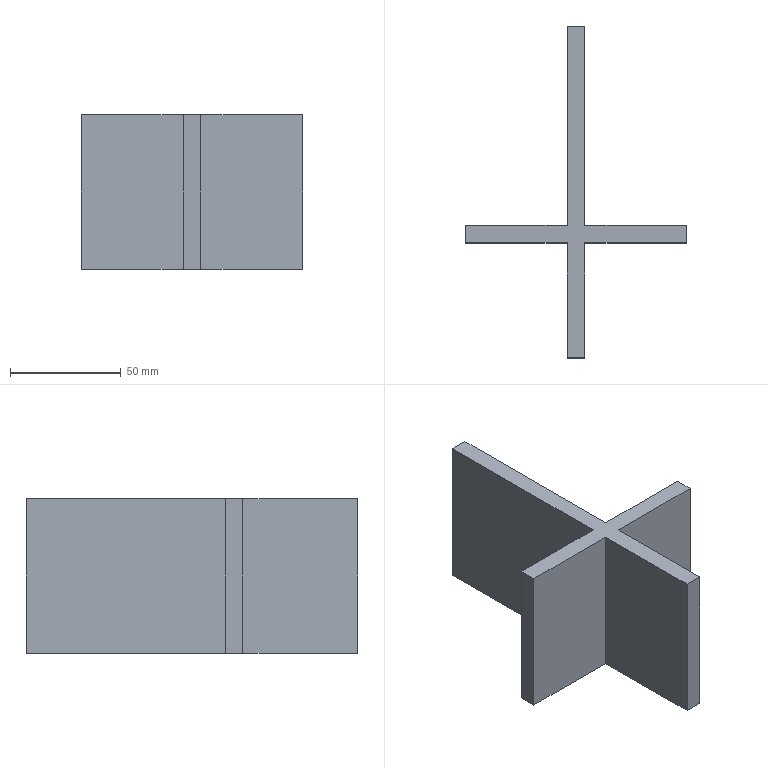Part | SolidWorks | features Extrusion 1 | 1 solid | 14 faces | box 100 x 150 x 70 mm | volume 135520 mm3 | plane 14
STEP:
#1=CARTESIAN_POINT('',(-50.,-4.,0.));
#2=VERTEX_POINT('',#1);
#3=CARTESIAN_POINT('',(-4.,-4.,0.));
#4=VERTEX_POINT('',#3);
#5=CARTESIAN_POINT('',(-4.,-4.,0.));
#6=DIRECTION('',(1.,0.,0.));
#7=VECTOR('',#6,1000.);
#8=LINE('',#5,#7);
#9=EDGE_CURVE('',#2,#4,#8,.T.);
#10=ORIENTED_EDGE('',*,*,#9,.T.);
#11=CARTESIAN_POINT('',(-4.,-4.,70.));
#12=VERTEX_POINT('',#11);
#13=CARTESIAN_POINT('',(-4.,-4.,70.));
#14=DIRECTION('',(0.,0.,-1.));
#15=VECTOR('',#14,1000.);
#16=LINE('',#13,#15);
#17=EDGE_CURVE('',#12,#4,#16,.T.);
#18=ORIENTED_EDGE('',*,*,#17,.F.);
#19=CARTESIAN_POINT('',(-50.,-4.,70.));
#20=VERTEX_POINT('',#19);
#21=CARTESIAN_POINT('',(-4.,-4.,70.));
#22=DIRECTION('',(1.,0.,0.));
#23=VECTOR('',#22,1000.);
#24=LINE('',#21,#23);
#25=EDGE_CURVE('',#20,#12,#24,.T.);
#26=ORIENTED_EDGE('',*,*,#25,.F.);
#27=CARTESIAN_POINT('',(-50.,-4.,70.));
#28=DIRECTION('',(0.,0.,-1.));
#29=VECTOR('',#28,1000.);
#30=LINE('',#27,#29);
#31=EDGE_CURVE('',#20,#2,#30,.T.);
#32=ORIENTED_EDGE('',*,*,#31,.T.);
#33=EDGE_LOOP('',(#10,#18,#26,#32));
#34=FACE_OUTER_BOUND('',#33,.T.);
#35=CARTESIAN_POINT('',(-4.,-4.,70.));
#36=DIRECTION('',(0.,1.,0.));
#37=DIRECTION('',(-1.,0.,0.));
#38=AXIS2_PLACEMENT_3D('',#35,#36,#37);
#39=PLANE('',#38);
#40=ADVANCED_FACE('',(#34),#39,.F.);
#41=CARTESIAN_POINT('',(-4.,-56.,0.));
#42=VERTEX_POINT('',#41);
#43=CARTESIAN_POINT('',(-4.,-4.,0.));
#44=DIRECTION('',(0.,-1.,0.));
#45=VECTOR('',#44,1000.);
#46=LINE('',#43,#45);
#47=EDGE_CURVE('',#4,#42,#46,.T.);
#48=ORIENTED_EDGE('',*,*,#47,.T.);
#49=CARTESIAN_POINT('',(-4.,-56.,70.));
#50=VERTEX_POINT('',#49);
#51=CARTESIAN_POINT('',(-4.,-56.,70.));
#52=DIRECTION('',(0.,0.,-1.));
#53=VECTOR('',#52,1000.);
#54=LINE('',#51,#53);
#55=EDGE_CURVE('',#50,#42,#54,.T.);
#56=ORIENTED_EDGE('',*,*,#55,.F.);
#57=CARTESIAN_POINT('',(-4.,-4.,70.));
#58=DIRECTION('',(0.,-1.,0.));
#59=VECTOR('',#58,1000.);
#60=LINE('',#57,#59);
#61=EDGE_CURVE('',#12,#50,#60,.T.);
#62=ORIENTED_EDGE('',*,*,#61,.F.);
#63=ORIENTED_EDGE('',*,*,#17,.T.);
#64=EDGE_LOOP('',(#48,#56,#62,#63));
#65=FACE_OUTER_BOUND('',#64,.T.);
#66=CARTESIAN_POINT('',(-4.,-4.,70.));
#67=DIRECTION('',(1.,0.,0.));
#68=DIRECTION('',(0.,0.,-1.));
#69=AXIS2_PLACEMENT_3D('',#66,#67,#68);
#70=PLANE('',#69);
#71=ADVANCED_FACE('',(#65),#70,.F.);
#72=CARTESIAN_POINT('',(4.,-56.,0.));
#73=VERTEX_POINT('',#72);
#74=CARTESIAN_POINT('',(4.,-56.,0.));
#75=DIRECTION('',(1.,0.,0.));
#76=VECTOR('',#75,1000.);
#77=LINE('',#74,#76);
#78=EDGE_CURVE('',#42,#73,#77,.T.);
#79=ORIENTED_EDGE('',*,*,#78,.T.);
#80=CARTESIAN_POINT('',(4.,-56.,70.));
#81=VERTEX_POINT('',#80);
#82=CARTESIAN_POINT('',(4.,-56.,70.));
#83=DIRECTION('',(0.,0.,-1.));
#84=VECTOR('',#83,1000.);
#85=LINE('',#82,#84);
#86=EDGE_CURVE('',#81,#73,#85,.T.);
#87=ORIENTED_EDGE('',*,*,#86,.F.);
#88=CARTESIAN_POINT('',(4.,-56.,70.));
#89=DIRECTION('',(1.,0.,0.));
#90=VECTOR('',#89,1000.);
#91=LINE('',#88,#90);
#92=EDGE_CURVE('',#50,#81,#91,.T.);
#93=ORIENTED_EDGE('',*,*,#92,.F.);
#94=ORIENTED_EDGE('',*,*,#55,.T.);
#95=EDGE_LOOP('',(#79,#87,#93,#94));
#96=FACE_OUTER_BOUND('',#95,.T.);
#97=CARTESIAN_POINT('',(4.,-56.,70.));
#98=DIRECTION('',(0.,1.,0.));
#99=DIRECTION('',(0.,0.,1.));
#100=AXIS2_PLACEMENT_3D('',#97,#98,#99);
#101=PLANE('',#100);
#102=ADVANCED_FACE('',(#96),#101,.F.);
#103=CARTESIAN_POINT('',(4.,-4.,0.));
#104=VERTEX_POINT('',#103);
#105=CARTESIAN_POINT('',(4.,-4.,0.));
#106=DIRECTION('',(0.,1.,0.));
#107=VECTOR('',#106,1000.);
#108=LINE('',#105,#107);
#109=EDGE_CURVE('',#73,#104,#108,.T.);
#110=ORIENTED_EDGE('',*,*,#109,.T.);
#111=CARTESIAN_POINT('',(4.,-4.,70.));
#112=VERTEX_POINT('',#111);
#113=CARTESIAN_POINT('',(4.,-4.,70.));
#114=DIRECTION('',(0.,0.,-1.));
#115=VECTOR('',#114,1000.);
#116=LINE('',#113,#115);
#117=EDGE_CURVE('',#112,#104,#116,.T.);
#118=ORIENTED_EDGE('',*,*,#117,.F.);
#119=CARTESIAN_POINT('',(4.,-4.,70.));
#120=DIRECTION('',(0.,1.,0.));
#121=VECTOR('',#120,1000.);
#122=LINE('',#119,#121);
#123=EDGE_CURVE('',#81,#112,#122,.T.);
#124=ORIENTED_EDGE('',*,*,#123,.F.);
#125=ORIENTED_EDGE('',*,*,#86,.T.);
#126=EDGE_LOOP('',(#110,#118,#124,#125));
#127=FACE_OUTER_BOUND('',#126,.T.);
#128=CARTESIAN_POINT('',(4.,-4.,70.));
#129=DIRECTION('',(-1.,0.,0.));
#130=DIRECTION('',(0.,-1.,0.));
#131=AXIS2_PLACEMENT_3D('',#128,#129,#130);
#132=PLANE('',#131);
#133=ADVANCED_FACE('',(#127),#132,.F.);
#134=CARTESIAN_POINT('',(50.,-4.,0.));
#135=VERTEX_POINT('',#134);
#136=CARTESIAN_POINT('',(50.,-4.,0.));
#137=DIRECTION('',(1.,0.,0.));
#138=VECTOR('',#137,1000.);
#139=LINE('',#136,#138);
#140=EDGE_CURVE('',#104,#135,#139,.T.);
#141=ORIENTED_EDGE('',*,*,#140,.T.);
#142=CARTESIAN_POINT('',(50.,-4.,70.));
#143=VERTEX_POINT('',#142);
#144=CARTESIAN_POINT('',(50.,-4.,70.));
#145=DIRECTION('',(0.,0.,-1.));
#146=VECTOR('',#145,1000.);
#147=LINE('',#144,#146);
#148=EDGE_CURVE('',#143,#135,#147,.T.);
#149=ORIENTED_EDGE('',*,*,#148,.F.);
#150=CARTESIAN_POINT('',(50.,-4.,70.));
#151=DIRECTION('',(1.,0.,0.));
#152=VECTOR('',#151,1000.);
#153=LINE('',#150,#152);
#154=EDGE_CURVE('',#112,#143,#153,.T.);
#155=ORIENTED_EDGE('',*,*,#154,.F.);
#156=ORIENTED_EDGE('',*,*,#117,.T.);
#157=EDGE_LOOP('',(#141,#149,#155,#156));
#158=FACE_OUTER_BOUND('',#157,.T.);
#159=CARTESIAN_POINT('',(50.,-4.,70.));
#160=DIRECTION('',(0.,1.,0.));
#161=DIRECTION('',(-1.,0.,0.));
#162=AXIS2_PLACEMENT_3D('',#159,#160,#161);
#163=PLANE('',#162);
#164=ADVANCED_FACE('',(#158),#163,.F.);
#165=CARTESIAN_POINT('',(50.,4.,0.));
#166=VERTEX_POINT('',#165);
#167=CARTESIAN_POINT('',(50.,4.,0.));
#168=DIRECTION('',(0.,1.,0.));
#169=VECTOR('',#168,1000.);
#170=LINE('',#167,#169);
#171=EDGE_CURVE('',#135,#166,#170,.T.);
#172=ORIENTED_EDGE('',*,*,#171,.T.);
#173=CARTESIAN_POINT('',(50.,4.,70.));
#174=VERTEX_POINT('',#173);
#175=CARTESIAN_POINT('',(50.,4.,70.));
#176=DIRECTION('',(0.,0.,-1.));
#177=VECTOR('',#176,1000.);
#178=LINE('',#175,#177);
#179=EDGE_CURVE('',#174,#166,#178,.T.);
#180=ORIENTED_EDGE('',*,*,#179,.F.);
#181=CARTESIAN_POINT('',(50.,4.,70.));
#182=DIRECTION('',(0.,1.,0.));
#183=VECTOR('',#182,1000.);
#184=LINE('',#181,#183);
#185=EDGE_CURVE('',#143,#174,#184,.T.);
#186=ORIENTED_EDGE('',*,*,#185,.F.);
#187=ORIENTED_EDGE('',*,*,#148,.T.);
#188=EDGE_LOOP('',(#172,#180,#186,#187));
#189=FACE_OUTER_BOUND('',#188,.T.);
#190=CARTESIAN_POINT('',(50.,4.,70.));
#191=DIRECTION('',(-1.,0.,0.));
#192=DIRECTION('',(0.,0.,1.));
#193=AXIS2_PLACEMENT_3D('',#190,#191,#192);
#194=PLANE('',#193);
#195=ADVANCED_FACE('',(#189),#194,.F.);
#196=CARTESIAN_POINT('',(4.,4.,0.));
#197=VERTEX_POINT('',#196);
#198=CARTESIAN_POINT('',(50.,4.,0.));
#199=DIRECTION('',(-1.,0.,0.));
#200=VECTOR('',#199,1000.);
#201=LINE('',#198,#200);
#202=EDGE_CURVE('',#166,#197,#201,.T.);
#203=ORIENTED_EDGE('',*,*,#202,.T.);
#204=CARTESIAN_POINT('',(4.,4.,70.));
#205=VERTEX_POINT('',#204);
#206=CARTESIAN_POINT('',(4.,4.,70.));
#207=DIRECTION('',(0.,0.,-1.));
#208=VECTOR('',#207,1000.);
#209=LINE('',#206,#208);
#210=EDGE_CURVE('',#205,#197,#209,.T.);
#211=ORIENTED_EDGE('',*,*,#210,.F.);
#212=CARTESIAN_POINT('',(50.,4.,70.));
#213=DIRECTION('',(-1.,0.,0.));
#214=VECTOR('',#213,1000.);
#215=LINE('',#212,#214);
#216=EDGE_CURVE('',#174,#205,#215,.T.);
#217=ORIENTED_EDGE('',*,*,#216,.F.);
#218=ORIENTED_EDGE('',*,*,#179,.T.);
#219=EDGE_LOOP('',(#203,#211,#217,#218));
#220=FACE_OUTER_BOUND('',#219,.T.);
#221=CARTESIAN_POINT('',(50.,4.,70.));
#222=DIRECTION('',(0.,-1.,0.));
#223=DIRECTION('',(1.,0.,0.));
#224=AXIS2_PLACEMENT_3D('',#221,#222,#223);
#225=PLANE('',#224);
#226=ADVANCED_FACE('',(#220),#225,.F.);
#227=CARTESIAN_POINT('',(4.,94.,0.));
#228=VERTEX_POINT('',#227);
#229=CARTESIAN_POINT('',(4.,94.,0.));
#230=DIRECTION('',(0.,1.,0.));
#231=VECTOR('',#230,1000.);
#232=LINE('',#229,#231);
#233=EDGE_CURVE('',#197,#228,#232,.T.);
#234=ORIENTED_EDGE('',*,*,#233,.T.);
#235=CARTESIAN_POINT('',(4.,94.,70.));
#236=VERTEX_POINT('',#235);
#237=CARTESIAN_POINT('',(4.,94.,70.));
#238=DIRECTION('',(0.,0.,-1.));
#239=VECTOR('',#238,1000.);
#240=LINE('',#237,#239);
#241=EDGE_CURVE('',#236,#228,#240,.T.);
#242=ORIENTED_EDGE('',*,*,#241,.F.);
#243=CARTESIAN_POINT('',(4.,94.,70.));
#244=DIRECTION('',(0.,1.,0.));
#245=VECTOR('',#244,1000.);
#246=LINE('',#243,#245);
#247=EDGE_CURVE('',#205,#236,#246,.T.);
#248=ORIENTED_EDGE('',*,*,#247,.F.);
#249=ORIENTED_EDGE('',*,*,#210,.T.);
#250=EDGE_LOOP('',(#234,#242,#248,#249));
#251=FACE_OUTER_BOUND('',#250,.T.);
#252=CARTESIAN_POINT('',(4.,94.,70.));
#253=DIRECTION('',(-1.,0.,0.));
#254=DIRECTION('',(0.,-1.,0.));
#255=AXIS2_PLACEMENT_3D('',#252,#253,#254);
#256=PLANE('',#255);
#257=ADVANCED_FACE('',(#251),#256,.F.);
#258=CARTESIAN_POINT('',(-4.,94.,0.));
#259=VERTEX_POINT('',#258);
#260=CARTESIAN_POINT('',(4.,94.,0.));
#261=DIRECTION('',(-1.,0.,0.));
#262=VECTOR('',#261,1000.);
#263=LINE('',#260,#262);
#264=EDGE_CURVE('',#228,#259,#263,.T.);
#265=ORIENTED_EDGE('',*,*,#264,.T.);
#266=CARTESIAN_POINT('',(-4.,94.,70.));
#267=VERTEX_POINT('',#266);
#268=CARTESIAN_POINT('',(-4.,94.,70.));
#269=DIRECTION('',(0.,0.,-1.));
#270=VECTOR('',#269,1000.);
#271=LINE('',#268,#270);
#272=EDGE_CURVE('',#267,#259,#271,.T.);
#273=ORIENTED_EDGE('',*,*,#272,.F.);
#274=CARTESIAN_POINT('',(4.,94.,70.));
#275=DIRECTION('',(-1.,0.,0.));
#276=VECTOR('',#275,1000.);
#277=LINE('',#274,#276);
#278=EDGE_CURVE('',#236,#267,#277,.T.);
#279=ORIENTED_EDGE('',*,*,#278,.F.);
#280=ORIENTED_EDGE('',*,*,#241,.T.);
#281=EDGE_LOOP('',(#265,#273,#279,#280));
#282=FACE_OUTER_BOUND('',#281,.T.);
#283=CARTESIAN_POINT('',(4.,94.,70.));
#284=DIRECTION('',(0.,-1.,0.));
#285=DIRECTION('',(0.,0.,-1.));
#286=AXIS2_PLACEMENT_3D('',#283,#284,#285);
#287=PLANE('',#286);
#288=ADVANCED_FACE('',(#282),#287,.F.);
#289=CARTESIAN_POINT('',(-4.,4.,0.));
#290=VERTEX_POINT('',#289);
#291=CARTESIAN_POINT('',(-4.,94.,0.));
#292=DIRECTION('',(0.,-1.,0.));
#293=VECTOR('',#292,1000.);
#294=LINE('',#291,#293);
#295=EDGE_CURVE('',#259,#290,#294,.T.);
#296=ORIENTED_EDGE('',*,*,#295,.T.);
#297=CARTESIAN_POINT('',(-4.,4.,70.));
#298=VERTEX_POINT('',#297);
#299=CARTESIAN_POINT('',(-4.,4.,70.));
#300=DIRECTION('',(0.,0.,-1.));
#301=VECTOR('',#300,1000.);
#302=LINE('',#299,#301);
#303=EDGE_CURVE('',#298,#290,#302,.T.);
#304=ORIENTED_EDGE('',*,*,#303,.F.);
#305=CARTESIAN_POINT('',(-4.,94.,70.));
#306=DIRECTION('',(0.,-1.,0.));
#307=VECTOR('',#306,1000.);
#308=LINE('',#305,#307);
#309=EDGE_CURVE('',#267,#298,#308,.T.);
#310=ORIENTED_EDGE('',*,*,#309,.F.);
#311=ORIENTED_EDGE('',*,*,#272,.T.);
#312=EDGE_LOOP('',(#296,#304,#310,#311));
#313=FACE_OUTER_BOUND('',#312,.T.);
#314=CARTESIAN_POINT('',(-4.,94.,70.));
#315=DIRECTION('',(1.,0.,0.));
#316=DIRECTION('',(0.,1.,0.));
#317=AXIS2_PLACEMENT_3D('',#314,#315,#316);
#318=PLANE('',#317);
#319=ADVANCED_FACE('',(#313),#318,.F.);
#320=CARTESIAN_POINT('',(-50.,4.,0.));
#321=VERTEX_POINT('',#320);
#322=CARTESIAN_POINT('',(-4.,4.,0.));
#323=DIRECTION('',(-1.,0.,0.));
#324=VECTOR('',#323,1000.);
#325=LINE('',#322,#324);
#326=EDGE_CURVE('',#290,#321,#325,.T.);
#327=ORIENTED_EDGE('',*,*,#326,.T.);
#328=CARTESIAN_POINT('',(-50.,4.,70.));
#329=VERTEX_POINT('',#328);
#330=CARTESIAN_POINT('',(-50.,4.,70.));
#331=DIRECTION('',(0.,0.,-1.));
#332=VECTOR('',#331,1000.);
#333=LINE('',#330,#332);
#334=EDGE_CURVE('',#329,#321,#333,.T.);
#335=ORIENTED_EDGE('',*,*,#334,.F.);
#336=CARTESIAN_POINT('',(-4.,4.,70.));
#337=DIRECTION('',(-1.,0.,0.));
#338=VECTOR('',#337,1000.);
#339=LINE('',#336,#338);
#340=EDGE_CURVE('',#298,#329,#339,.T.);
#341=ORIENTED_EDGE('',*,*,#340,.F.);
#342=ORIENTED_EDGE('',*,*,#303,.T.);
#343=EDGE_LOOP('',(#327,#335,#341,#342));
#344=FACE_OUTER_BOUND('',#343,.T.);
#345=CARTESIAN_POINT('',(-4.,4.,70.));
#346=DIRECTION('',(0.,-1.,0.));
#347=DIRECTION('',(1.,0.,0.));
#348=AXIS2_PLACEMENT_3D('',#345,#346,#347);
#349=PLANE('',#348);
#350=ADVANCED_FACE('',(#344),#349,.F.);
#351=CARTESIAN_POINT('',(-50.,4.,0.));
#352=DIRECTION('',(0.,-1.,0.));
#353=VECTOR('',#352,1000.);
#354=LINE('',#351,#353);
#355=EDGE_CURVE('',#321,#2,#354,.T.);
#356=ORIENTED_EDGE('',*,*,#355,.T.);
#357=ORIENTED_EDGE('',*,*,#31,.F.);
#358=CARTESIAN_POINT('',(-50.,4.,70.));
#359=DIRECTION('',(0.,-1.,0.));
#360=VECTOR('',#359,1000.);
#361=LINE('',#358,#360);
#362=EDGE_CURVE('',#329,#20,#361,.T.);
#363=ORIENTED_EDGE('',*,*,#362,.F.);
#364=ORIENTED_EDGE('',*,*,#334,.T.);
#365=EDGE_LOOP('',(#356,#357,#363,#364));
#366=FACE_OUTER_BOUND('',#365,.T.);
#367=CARTESIAN_POINT('',(-50.,4.,70.));
#368=DIRECTION('',(1.,0.,0.));
#369=DIRECTION('',(0.,0.,-1.));
#370=AXIS2_PLACEMENT_3D('',#367,#368,#369);
#371=PLANE('',#370);
#372=ADVANCED_FACE('',(#366),#371,.F.);
#373=ORIENTED_EDGE('',*,*,#25,.T.);
#374=ORIENTED_EDGE('',*,*,#61,.T.);
#375=ORIENTED_EDGE('',*,*,#92,.T.);
#376=ORIENTED_EDGE('',*,*,#123,.T.);
#377=ORIENTED_EDGE('',*,*,#154,.T.);
#378=ORIENTED_EDGE('',*,*,#185,.T.);
#379=ORIENTED_EDGE('',*,*,#216,.T.);
#380=ORIENTED_EDGE('',*,*,#247,.T.);
#381=ORIENTED_EDGE('',*,*,#278,.T.);
#382=ORIENTED_EDGE('',*,*,#309,.T.);
#383=ORIENTED_EDGE('',*,*,#340,.T.);
#384=ORIENTED_EDGE('',*,*,#362,.T.);
#385=EDGE_LOOP('',(#373,#374,#375,#376,#377,#378,#379,#380,#381,#382,#383,#384));
#386=FACE_OUTER_BOUND('',#385,.T.);
#387=CARTESIAN_POINT('',(0.,0.,70.));
#388=DIRECTION('',(0.,0.,1.));
#389=DIRECTION('',(1.,0.,0.));
#390=AXIS2_PLACEMENT_3D('',#387,#388,#389);
#391=PLANE('',#390);
#392=ADVANCED_FACE('',(#386),#391,.T.);
#393=ORIENTED_EDGE('',*,*,#9,.F.);
#394=ORIENTED_EDGE('',*,*,#355,.F.);
#395=ORIENTED_EDGE('',*,*,#326,.F.);
#396=ORIENTED_EDGE('',*,*,#295,.F.);
#397=ORIENTED_EDGE('',*,*,#264,.F.);
#398=ORIENTED_EDGE('',*,*,#233,.F.);
#399=ORIENTED_EDGE('',*,*,#202,.F.);
#400=ORIENTED_EDGE('',*,*,#171,.F.);
#401=ORIENTED_EDGE('',*,*,#140,.F.);
#402=ORIENTED_EDGE('',*,*,#109,.F.);
#403=ORIENTED_EDGE('',*,*,#78,.F.);
#404=ORIENTED_EDGE('',*,*,#47,.F.);
#405=EDGE_LOOP('',(#393,#394,#395,#396,#397,#398,#399,#400,#401,#402,#403,#404));
#406=FACE_OUTER_BOUND('',#405,.T.);
#407=CARTESIAN_POINT('',(0.,0.,0.));
#408=DIRECTION('',(0.,0.,1.));
#409=DIRECTION('',(1.,0.,0.));
#410=AXIS2_PLACEMENT_3D('',#407,#408,#409);
#411=PLANE('',#410);
#412=ADVANCED_FACE('',(#406),#411,.F.);
#413=CLOSED_SHELL('',(#40,#71,#102,#133,#164,#195,#226,#257,#288,#319,#350,#372,#392,#412));
#414=MANIFOLD_SOLID_BREP('',#413);
#415=CARTESIAN_POINT('',(0.,0.,0.));
#416=DIRECTION('',(0.,0.,1.));
#417=DIRECTION('',(1.,0.,0.));
#418=AXIS2_PLACEMENT_3D('',#415,#416,#417);
#419=(LENGTH_UNIT()NAMED_UNIT(*)SI_UNIT(.MILLI.,.METRE.));
#420=UNCERTAINTY_MEASURE_WITH_UNIT(LENGTH_MEASURE(0.00001),#419,'','');
#421=(NAMED_UNIT(*)PLANE_ANGLE_UNIT()SI_UNIT($,.RADIAN.));
#422=(NAMED_UNIT(*)SI_UNIT($,.STERADIAN.)SOLID_ANGLE_UNIT());
#423=(GEOMETRIC_REPRESENTATION_CONTEXT(3)GLOBAL_UNCERTAINTY_ASSIGNED_CONTEXT((#420))GLOBAL_UNIT_ASSIGNED_CONTEXT((#419,#421,#422))REPRESENTATION_CONTEXT('',''));
#424=ADVANCED_BREP_SHAPE_REPRESENTATION('',(#414,#418),#423);